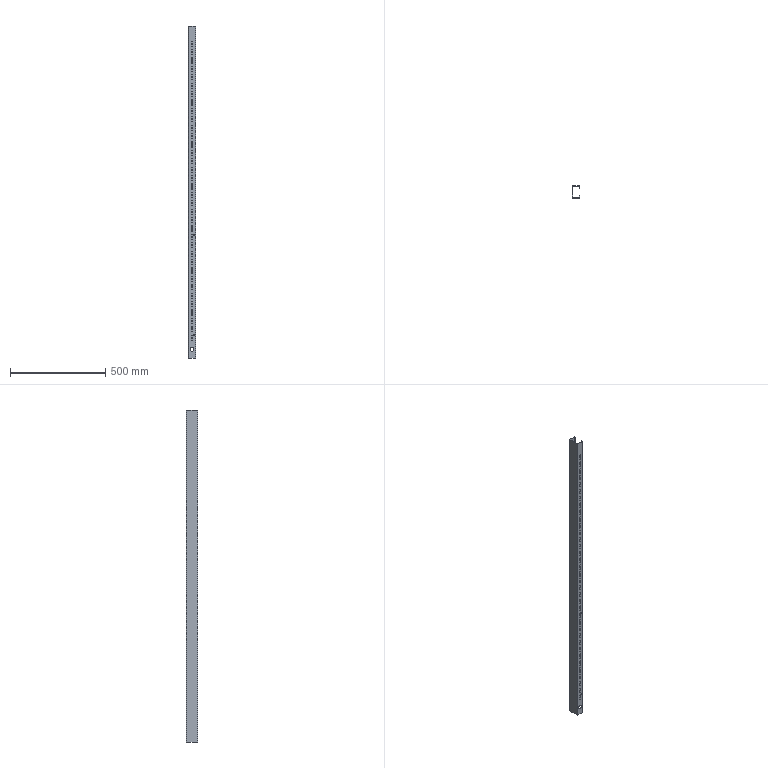Part | STEP file | 1 solid | 618 faces | box 37 x 60 x 1739 mm | volume 359909 mm3 | plane 310 | cylinder 308 | commonest cylinder face diameters 3 x144 6.5 x144 0.4 x4 3.4 x4 5.1 x4 6.3 x4